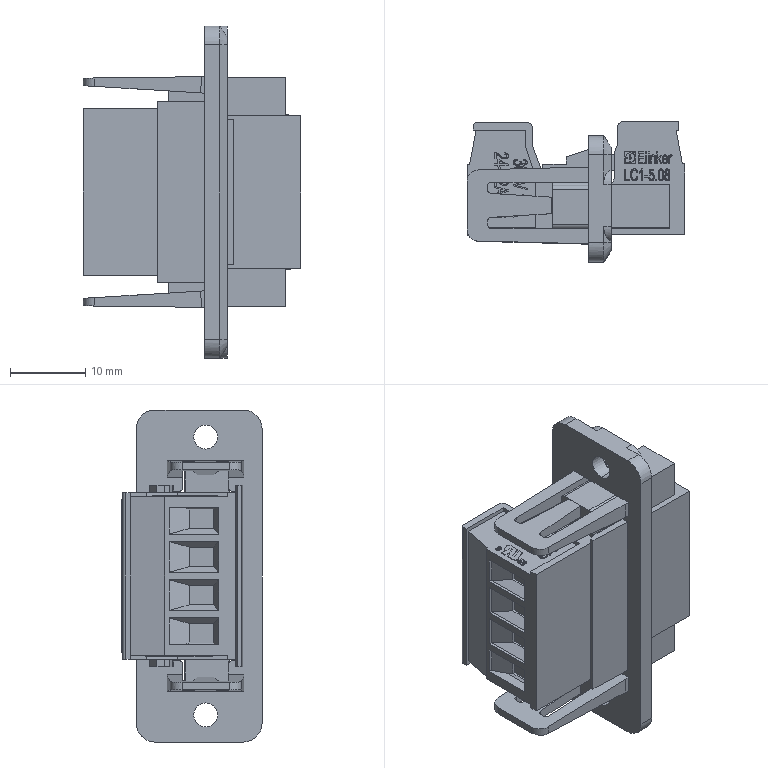Part | NX | features BREP 21 | 21 solids | 7625 faces | volume 9257 mm3 | plane 6884 | cylinder 319 | spline 302 | torus 88 | cone 32 | commonest cylinder face diameters 3.2 x48 3.6 x36 2.5 x22 3.9 x20 4 x20 1.2 x12